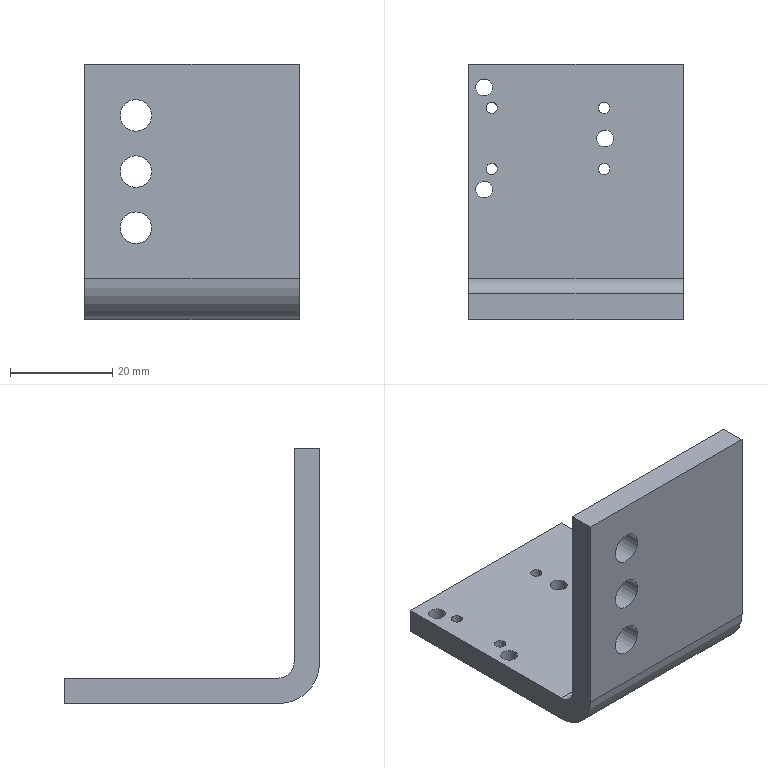Part | NX | features SIMPLE HOLE 10, DATUM_CSYS 5, SKETCH 4, HOLE PACKAGE 3, EXTRUDE 1 | 1 solid | 20 faces | box 42 x 50 x 50 mm | volume 18797 mm3 | cylinder 12 | plane 8 | commonest cylinder face diameters 2.2 x4 3.3 x3 6.2 x3 6 x1 16 x1
STEP:
#1=CARTESIAN_POINT('',(-11.,0.,43.1));
#2=VERTEX_POINT('',#1);
#3=CARTESIAN_POINT('',(-11.,0.,40.));
#4=DIRECTION('',(0.,1.,0.));
#5=DIRECTION('',(0.,0.,1.));
#6=AXIS2_PLACEMENT_3D('',#3,#4,#5);
#7=CIRCLE('',#6,3.1);
#8=EDGE_CURVE('',#2,#2,#7,.T.);
#9=ORIENTED_EDGE('',*,*,#8,.T.);
#10=EDGE_LOOP('',(#9));
#11=FACE_BOUND('',#10,.T.);
#12=CARTESIAN_POINT('',(-11.,0.,32.1));
#13=VERTEX_POINT('',#12);
#14=CARTESIAN_POINT('',(-11.,0.,29.));
#15=DIRECTION('',(0.,1.,0.));
#16=DIRECTION('',(0.,0.,1.));
#17=AXIS2_PLACEMENT_3D('',#14,#15,#16);
#18=CIRCLE('',#17,3.1);
#19=EDGE_CURVE('',#13,#13,#18,.T.);
#20=ORIENTED_EDGE('',*,*,#19,.T.);
#21=EDGE_LOOP('',(#20));
#22=FACE_BOUND('',#21,.T.);
#23=CARTESIAN_POINT('',(-11.,0.,21.1));
#24=VERTEX_POINT('',#23);
#25=CARTESIAN_POINT('',(-11.,0.,18.));
#26=DIRECTION('',(0.,1.,0.));
#27=DIRECTION('',(0.,0.,1.));
#28=AXIS2_PLACEMENT_3D('',#25,#26,#27);
#29=CIRCLE('',#28,3.1);
#30=EDGE_CURVE('',#24,#24,#29,.T.);
#31=ORIENTED_EDGE('',*,*,#30,.T.);
#32=EDGE_LOOP('',(#31));
#33=FACE_BOUND('',#32,.T.);
#34=CARTESIAN_POINT('',(-21.,0.,50.));
#35=VERTEX_POINT('',#34);
#36=CARTESIAN_POINT('',(-21.,0.,8.));
#37=VERTEX_POINT('',#36);
#38=CARTESIAN_POINT('',(-21.,0.,50.));
#39=DIRECTION('',(0.,0.,-1.));
#40=VECTOR('',#39,1000.);
#41=LINE('',#38,#40);
#42=EDGE_CURVE('',#35,#37,#41,.T.);
#43=ORIENTED_EDGE('',*,*,#42,.T.);
#44=CARTESIAN_POINT('',(21.,0.,8.));
#45=VERTEX_POINT('',#44);
#46=CARTESIAN_POINT('',(21.,0.,8.));
#47=DIRECTION('',(-1.,0.,0.));
#48=VECTOR('',#47,1000.);
#49=LINE('',#46,#48);
#50=EDGE_CURVE('',#45,#37,#49,.T.);
#51=ORIENTED_EDGE('',*,*,#50,.F.);
#52=CARTESIAN_POINT('',(21.,0.,50.));
#53=VERTEX_POINT('',#52);
#54=CARTESIAN_POINT('',(21.,0.,50.));
#55=DIRECTION('',(0.,0.,-1.));
#56=VECTOR('',#55,1000.);
#57=LINE('',#54,#56);
#58=EDGE_CURVE('',#53,#45,#57,.T.);
#59=ORIENTED_EDGE('',*,*,#58,.F.);
#60=CARTESIAN_POINT('',(21.,0.,50.));
#61=DIRECTION('',(-1.,0.,0.));
#62=VECTOR('',#61,1000.);
#63=LINE('',#60,#62);
#64=EDGE_CURVE('',#53,#35,#63,.T.);
#65=ORIENTED_EDGE('',*,*,#64,.T.);
#66=EDGE_LOOP('',(#43,#51,#59,#65));
#67=FACE_BOUND('',#66,.T.);
#68=CARTESIAN_POINT('',(21.,0.,50.));
#69=DIRECTION('',(0.,1.,0.));
#70=DIRECTION('',(0.,0.,1.));
#71=AXIS2_PLACEMENT_3D('',#68,#69,#70);
#72=PLANE('',#71);
#73=ADVANCED_FACE('',(#11,#22,#33,#67),#72,.F.);
#74=CARTESIAN_POINT('',(-21.,8.,0.));
#75=VERTEX_POINT('',#74);
#76=CARTESIAN_POINT('',(-21.,8.,8.));
#77=DIRECTION('',(1.,0.,0.));
#78=DIRECTION('',(0.,1.,0.));
#79=AXIS2_PLACEMENT_3D('',#76,#77,#78);
#80=CIRCLE('',#79,8.);
#81=EDGE_CURVE('',#37,#75,#80,.T.);
#82=ORIENTED_EDGE('',*,*,#81,.T.);
#83=CARTESIAN_POINT('',(21.,8.,0.));
#84=VERTEX_POINT('',#83);
#85=CARTESIAN_POINT('',(21.,8.,0.));
#86=DIRECTION('',(-1.,0.,0.));
#87=VECTOR('',#86,1000.);
#88=LINE('',#85,#87);
#89=EDGE_CURVE('',#84,#75,#88,.T.);
#90=ORIENTED_EDGE('',*,*,#89,.F.);
#91=CARTESIAN_POINT('',(21.,8.,8.));
#92=DIRECTION('',(1.,0.,0.));
#93=DIRECTION('',(0.,1.,0.));
#94=AXIS2_PLACEMENT_3D('',#91,#92,#93);
#95=CIRCLE('',#94,8.);
#96=EDGE_CURVE('',#45,#84,#95,.T.);
#97=ORIENTED_EDGE('',*,*,#96,.F.);
#98=ORIENTED_EDGE('',*,*,#50,.T.);
#99=EDGE_LOOP('',(#82,#90,#97,#98));
#100=FACE_BOUND('',#99,.T.);
#101=CARTESIAN_POINT('',(21.,8.,8.));
#102=DIRECTION('',(-1.,0.,0.));
#103=DIRECTION('',(0.,0.,1.));
#104=AXIS2_PLACEMENT_3D('',#101,#102,#103);
#105=CYLINDRICAL_SURFACE('',#104,8.);
#106=ADVANCED_FACE('',(#100),#105,.T.);
#107=CARTESIAN_POINT('',(6.6,41.5,0.));
#108=VERTEX_POINT('',#107);
#109=CARTESIAN_POINT('',(5.5,41.5,0.));
#110=DIRECTION('',(0.,0.,1.));
#111=DIRECTION('',(1.,0.,0.));
#112=AXIS2_PLACEMENT_3D('',#109,#110,#111);
#113=CIRCLE('',#112,1.1);
#114=EDGE_CURVE('',#108,#108,#113,.T.);
#115=ORIENTED_EDGE('',*,*,#114,.T.);
#116=EDGE_LOOP('',(#115));
#117=FACE_BOUND('',#116,.T.);
#118=CARTESIAN_POINT('',(6.6,29.5,0.));
#119=VERTEX_POINT('',#118);
#120=CARTESIAN_POINT('',(5.5,29.5,0.));
#121=DIRECTION('',(0.,0.,1.));
#122=DIRECTION('',(1.,0.,0.));
#123=AXIS2_PLACEMENT_3D('',#120,#121,#122);
#124=CIRCLE('',#123,1.1);
#125=EDGE_CURVE('',#119,#119,#124,.T.);
#126=ORIENTED_EDGE('',*,*,#125,.T.);
#127=EDGE_LOOP('',(#126));
#128=FACE_BOUND('',#127,.T.);
#129=CARTESIAN_POINT('',(-15.4,41.5,0.));
#130=VERTEX_POINT('',#129);
#131=CARTESIAN_POINT('',(-16.5,41.5,0.));
#132=DIRECTION('',(0.,0.,1.));
#133=DIRECTION('',(1.,0.,0.));
#134=AXIS2_PLACEMENT_3D('',#131,#132,#133);
#135=CIRCLE('',#134,1.1);
#136=EDGE_CURVE('',#130,#130,#135,.T.);
#137=ORIENTED_EDGE('',*,*,#136,.T.);
#138=EDGE_LOOP('',(#137));
#139=FACE_BOUND('',#138,.T.);
#140=CARTESIAN_POINT('',(-15.4,29.5,0.));
#141=VERTEX_POINT('',#140);
#142=CARTESIAN_POINT('',(-16.5,29.5,0.));
#143=DIRECTION('',(0.,0.,1.));
#144=DIRECTION('',(1.,0.,0.));
#145=AXIS2_PLACEMENT_3D('',#142,#143,#144);
#146=CIRCLE('',#145,1.1);
#147=EDGE_CURVE('',#141,#141,#146,.T.);
#148=ORIENTED_EDGE('',*,*,#147,.T.);
#149=EDGE_LOOP('',(#148));
#150=FACE_BOUND('',#149,.T.);
#151=CARTESIAN_POINT('',(7.35,35.5,0.));
#152=VERTEX_POINT('',#151);
#153=CARTESIAN_POINT('',(5.7,35.5,0.));
#154=DIRECTION('',(0.,0.,1.));
#155=DIRECTION('',(1.,0.,0.));
#156=AXIS2_PLACEMENT_3D('',#153,#154,#155);
#157=CIRCLE('',#156,1.65);
#158=EDGE_CURVE('',#152,#152,#157,.T.);
#159=ORIENTED_EDGE('',*,*,#158,.T.);
#160=EDGE_LOOP('',(#159));
#161=FACE_BOUND('',#160,.T.);
#162=CARTESIAN_POINT('',(-16.35,45.5,0.));
#163=VERTEX_POINT('',#162);
#164=CARTESIAN_POINT('',(-18.,45.5,0.));
#165=DIRECTION('',(0.,0.,1.));
#166=DIRECTION('',(1.,0.,0.));
#167=AXIS2_PLACEMENT_3D('',#164,#165,#166);
#168=CIRCLE('',#167,1.65);
#169=EDGE_CURVE('',#163,#163,#168,.T.);
#170=ORIENTED_EDGE('',*,*,#169,.T.);
#171=EDGE_LOOP('',(#170));
#172=FACE_BOUND('',#171,.T.);
#173=CARTESIAN_POINT('',(-16.35,25.5,0.));
#174=VERTEX_POINT('',#173);
#175=CARTESIAN_POINT('',(-18.,25.5,0.));
#176=DIRECTION('',(0.,0.,1.));
#177=DIRECTION('',(1.,0.,0.));
#178=AXIS2_PLACEMENT_3D('',#175,#176,#177);
#179=CIRCLE('',#178,1.65);
#180=EDGE_CURVE('',#174,#174,#179,.T.);
#181=ORIENTED_EDGE('',*,*,#180,.T.);
#182=EDGE_LOOP('',(#181));
#183=FACE_BOUND('',#182,.T.);
#184=CARTESIAN_POINT('',(-21.,50.,0.));
#185=VERTEX_POINT('',#184);
#186=CARTESIAN_POINT('',(-21.,8.,0.));
#187=DIRECTION('',(0.,1.,0.));
#188=VECTOR('',#187,1000.);
#189=LINE('',#186,#188);
#190=EDGE_CURVE('',#75,#185,#189,.T.);
#191=ORIENTED_EDGE('',*,*,#190,.T.);
#192=CARTESIAN_POINT('',(21.,50.,0.));
#193=VERTEX_POINT('',#192);
#194=CARTESIAN_POINT('',(21.,50.,0.));
#195=DIRECTION('',(-1.,0.,0.));
#196=VECTOR('',#195,1000.);
#197=LINE('',#194,#196);
#198=EDGE_CURVE('',#193,#185,#197,.T.);
#199=ORIENTED_EDGE('',*,*,#198,.F.);
#200=CARTESIAN_POINT('',(21.,8.,0.));
#201=DIRECTION('',(0.,1.,0.));
#202=VECTOR('',#201,1000.);
#203=LINE('',#200,#202);
#204=EDGE_CURVE('',#84,#193,#203,.T.);
#205=ORIENTED_EDGE('',*,*,#204,.F.);
#206=ORIENTED_EDGE('',*,*,#89,.T.);
#207=EDGE_LOOP('',(#191,#199,#205,#206));
#208=FACE_BOUND('',#207,.T.);
#209=CARTESIAN_POINT('',(21.,8.,0.));
#210=DIRECTION('',(0.,0.,1.));
#211=DIRECTION('',(1.,0.,0.));
#212=AXIS2_PLACEMENT_3D('',#209,#210,#211);
#213=PLANE('',#212);
#214=ADVANCED_FACE('',(#117,#128,#139,#150,#161,#172,#183,#208),#213,.F.);
#215=CARTESIAN_POINT('',(-21.,50.,5.));
#216=VERTEX_POINT('',#215);
#217=CARTESIAN_POINT('',(-21.,50.,0.));
#218=DIRECTION('',(0.,0.,1.));
#219=VECTOR('',#218,1000.);
#220=LINE('',#217,#219);
#221=EDGE_CURVE('',#185,#216,#220,.T.);
#222=ORIENTED_EDGE('',*,*,#221,.T.);
#223=CARTESIAN_POINT('',(21.,50.,5.));
#224=VERTEX_POINT('',#223);
#225=CARTESIAN_POINT('',(21.,50.,5.));
#226=DIRECTION('',(-1.,0.,0.));
#227=VECTOR('',#226,1000.);
#228=LINE('',#225,#227);
#229=EDGE_CURVE('',#224,#216,#228,.T.);
#230=ORIENTED_EDGE('',*,*,#229,.F.);
#231=CARTESIAN_POINT('',(21.,50.,0.));
#232=DIRECTION('',(0.,0.,1.));
#233=VECTOR('',#232,1000.);
#234=LINE('',#231,#233);
#235=EDGE_CURVE('',#193,#224,#234,.T.);
#236=ORIENTED_EDGE('',*,*,#235,.F.);
#237=ORIENTED_EDGE('',*,*,#198,.T.);
#238=EDGE_LOOP('',(#222,#230,#236,#237));
#239=FACE_BOUND('',#238,.T.);
#240=CARTESIAN_POINT('',(21.,50.,0.));
#241=DIRECTION('',(0.,-1.,0.));
#242=DIRECTION('',(0.,0.,-1.));
#243=AXIS2_PLACEMENT_3D('',#240,#241,#242);
#244=PLANE('',#243);
#245=ADVANCED_FACE('',(#239),#244,.F.);
#246=CARTESIAN_POINT('',(5.5,42.6,5.));
#247=VERTEX_POINT('',#246);
#248=CARTESIAN_POINT('',(5.5,41.5,5.));
#249=DIRECTION('',(0.,0.,-1.));
#250=DIRECTION('',(0.,1.,0.));
#251=AXIS2_PLACEMENT_3D('',#248,#249,#250);
#252=CIRCLE('',#251,1.1);
#253=EDGE_CURVE('',#247,#247,#252,.T.);
#254=ORIENTED_EDGE('',*,*,#253,.T.);
#255=EDGE_LOOP('',(#254));
#256=FACE_BOUND('',#255,.T.);
#257=CARTESIAN_POINT('',(5.5,30.6,5.));
#258=VERTEX_POINT('',#257);
#259=CARTESIAN_POINT('',(5.5,29.5,5.));
#260=DIRECTION('',(0.,0.,-1.));
#261=DIRECTION('',(0.,1.,0.));
#262=AXIS2_PLACEMENT_3D('',#259,#260,#261);
#263=CIRCLE('',#262,1.1);
#264=EDGE_CURVE('',#258,#258,#263,.T.);
#265=ORIENTED_EDGE('',*,*,#264,.T.);
#266=EDGE_LOOP('',(#265));
#267=FACE_BOUND('',#266,.T.);
#268=CARTESIAN_POINT('',(-16.5,42.6,5.));
#269=VERTEX_POINT('',#268);
#270=CARTESIAN_POINT('',(-16.5,41.5,5.));
#271=DIRECTION('',(0.,0.,-1.));
#272=DIRECTION('',(0.,1.,0.));
#273=AXIS2_PLACEMENT_3D('',#270,#271,#272);
#274=CIRCLE('',#273,1.1);
#275=EDGE_CURVE('',#269,#269,#274,.T.);
#276=ORIENTED_EDGE('',*,*,#275,.T.);
#277=EDGE_LOOP('',(#276));
#278=FACE_BOUND('',#277,.T.);
#279=CARTESIAN_POINT('',(-16.5,30.6,5.));
#280=VERTEX_POINT('',#279);
#281=CARTESIAN_POINT('',(-16.5,29.5,5.));
#282=DIRECTION('',(0.,0.,-1.));
#283=DIRECTION('',(0.,1.,0.));
#284=AXIS2_PLACEMENT_3D('',#281,#282,#283);
#285=CIRCLE('',#284,1.1);
#286=EDGE_CURVE('',#280,#280,#285,.T.);
#287=ORIENTED_EDGE('',*,*,#286,.T.);
#288=EDGE_LOOP('',(#287));
#289=FACE_BOUND('',#288,.T.);
#290=CARTESIAN_POINT('',(5.7,37.15,5.));
#291=VERTEX_POINT('',#290);
#292=CARTESIAN_POINT('',(5.7,35.5,5.));
#293=DIRECTION('',(0.,0.,-1.));
#294=DIRECTION('',(0.,1.,0.));
#295=AXIS2_PLACEMENT_3D('',#292,#293,#294);
#296=CIRCLE('',#295,1.65);
#297=EDGE_CURVE('',#291,#291,#296,.T.);
#298=ORIENTED_EDGE('',*,*,#297,.T.);
#299=EDGE_LOOP('',(#298));
#300=FACE_BOUND('',#299,.T.);
#301=CARTESIAN_POINT('',(-18.,47.15,5.));
#302=VERTEX_POINT('',#301);
#303=CARTESIAN_POINT('',(-18.,45.5,5.));
#304=DIRECTION('',(0.,0.,-1.));
#305=DIRECTION('',(0.,1.,0.));
#306=AXIS2_PLACEMENT_3D('',#303,#304,#305);
#307=CIRCLE('',#306,1.65);
#308=EDGE_CURVE('',#302,#302,#307,.T.);
#309=ORIENTED_EDGE('',*,*,#308,.T.);
#310=EDGE_LOOP('',(#309));
#311=FACE_BOUND('',#310,.T.);
#312=CARTESIAN_POINT('',(-18.,27.15,5.));
#313=VERTEX_POINT('',#312);
#314=CARTESIAN_POINT('',(-18.,25.5,5.));
#315=DIRECTION('',(0.,0.,-1.));
#316=DIRECTION('',(0.,1.,0.));
#317=AXIS2_PLACEMENT_3D('',#314,#315,#316);
#318=CIRCLE('',#317,1.65);
#319=EDGE_CURVE('',#313,#313,#318,.T.);
#320=ORIENTED_EDGE('',*,*,#319,.T.);
#321=EDGE_LOOP('',(#320));
#322=FACE_BOUND('',#321,.T.);
#323=CARTESIAN_POINT('',(-21.,8.,5.));
#324=VERTEX_POINT('',#323);
#325=CARTESIAN_POINT('',(-21.,50.,5.));
#326=DIRECTION('',(0.,-1.,0.));
#327=VECTOR('',#326,1000.);
#328=LINE('',#325,#327);
#329=EDGE_CURVE('',#216,#324,#328,.T.);
#330=ORIENTED_EDGE('',*,*,#329,.T.);
#331=CARTESIAN_POINT('',(21.,8.,5.));
#332=VERTEX_POINT('',#331);
#333=CARTESIAN_POINT('',(21.,8.,5.));
#334=DIRECTION('',(-1.,0.,0.));
#335=VECTOR('',#334,1000.);
#336=LINE('',#333,#335);
#337=EDGE_CURVE('',#332,#324,#336,.T.);
#338=ORIENTED_EDGE('',*,*,#337,.F.);
#339=CARTESIAN_POINT('',(21.,50.,5.));
#340=DIRECTION('',(0.,-1.,0.));
#341=VECTOR('',#340,1000.);
#342=LINE('',#339,#341);
#343=EDGE_CURVE('',#224,#332,#342,.T.);
#344=ORIENTED_EDGE('',*,*,#343,.F.);
#345=ORIENTED_EDGE('',*,*,#229,.T.);
#346=EDGE_LOOP('',(#330,#338,#344,#345));
#347=FACE_BOUND('',#346,.T.);
#348=CARTESIAN_POINT('',(21.,50.,5.));
#349=DIRECTION('',(0.,0.,-1.));
#350=DIRECTION('',(0.,1.,0.));
#351=AXIS2_PLACEMENT_3D('',#348,#349,#350);
#352=PLANE('',#351);
#353=ADVANCED_FACE('',(#256,#267,#278,#289,#300,#311,#322,#347),#352,.F.);
#354=CARTESIAN_POINT('',(-21.,5.,8.));
#355=VERTEX_POINT('',#354);
#356=CARTESIAN_POINT('',(-21.,8.,8.));
#357=DIRECTION('',(-1.,0.,0.));
#358=DIRECTION('',(0.,1.,0.));
#359=AXIS2_PLACEMENT_3D('',#356,#357,#358);
#360=CIRCLE('',#359,3.);
#361=EDGE_CURVE('',#324,#355,#360,.T.);
#362=ORIENTED_EDGE('',*,*,#361,.T.);
#363=CARTESIAN_POINT('',(21.,5.,8.));
#364=VERTEX_POINT('',#363);
#365=CARTESIAN_POINT('',(21.,5.,8.));
#366=DIRECTION('',(-1.,0.,0.));
#367=VECTOR('',#366,1000.);
#368=LINE('',#365,#367);
#369=EDGE_CURVE('',#364,#355,#368,.T.);
#370=ORIENTED_EDGE('',*,*,#369,.F.);
#371=CARTESIAN_POINT('',(21.,8.,8.));
#372=DIRECTION('',(-1.,0.,0.));
#373=DIRECTION('',(0.,1.,0.));
#374=AXIS2_PLACEMENT_3D('',#371,#372,#373);
#375=CIRCLE('',#374,3.);
#376=EDGE_CURVE('',#332,#364,#375,.T.);
#377=ORIENTED_EDGE('',*,*,#376,.F.);
#378=ORIENTED_EDGE('',*,*,#337,.T.);
#379=EDGE_LOOP('',(#362,#370,#377,#378));
#380=FACE_BOUND('',#379,.T.);
#381=CARTESIAN_POINT('',(21.,8.,8.));
#382=DIRECTION('',(-1.,0.,0.));
#383=DIRECTION('',(0.,0.,1.));
#384=AXIS2_PLACEMENT_3D('',#381,#382,#383);
#385=CYLINDRICAL_SURFACE('',#384,3.);
#386=ADVANCED_FACE('',(#380),#385,.F.);
#387=CARTESIAN_POINT('',(-11.,5.,36.9));
#388=VERTEX_POINT('',#387);
#389=CARTESIAN_POINT('',(-11.,5.,40.));
#390=DIRECTION('',(0.,-1.,0.));
#391=DIRECTION('',(0.,0.,-1.));
#392=AXIS2_PLACEMENT_3D('',#389,#390,#391);
#393=CIRCLE('',#392,3.1);
#394=EDGE_CURVE('',#388,#388,#393,.T.);
#395=ORIENTED_EDGE('',*,*,#394,.T.);
#396=EDGE_LOOP('',(#395));
#397=FACE_BOUND('',#396,.T.);
#398=CARTESIAN_POINT('',(-11.,5.,25.9));
#399=VERTEX_POINT('',#398);
#400=CARTESIAN_POINT('',(-11.,5.,29.));
#401=DIRECTION('',(0.,-1.,0.));
#402=DIRECTION('',(0.,0.,-1.));
#403=AXIS2_PLACEMENT_3D('',#400,#401,#402);
#404=CIRCLE('',#403,3.1);
#405=EDGE_CURVE('',#399,#399,#404,.T.);
#406=ORIENTED_EDGE('',*,*,#405,.T.);
#407=EDGE_LOOP('',(#406));
#408=FACE_BOUND('',#407,.T.);
#409=CARTESIAN_POINT('',(-11.,5.,14.9));
#410=VERTEX_POINT('',#409);
#411=CARTESIAN_POINT('',(-11.,5.,18.));
#412=DIRECTION('',(0.,-1.,0.));
#413=DIRECTION('',(0.,0.,-1.));
#414=AXIS2_PLACEMENT_3D('',#411,#412,#413);
#415=CIRCLE('',#414,3.1);
#416=EDGE_CURVE('',#410,#410,#415,.T.);
#417=ORIENTED_EDGE('',*,*,#416,.T.);
#418=EDGE_LOOP('',(#417));
#419=FACE_BOUND('',#418,.T.);
#420=CARTESIAN_POINT('',(-21.,5.,50.));
#421=VERTEX_POINT('',#420);
#422=CARTESIAN_POINT('',(-21.,5.,8.));
#423=DIRECTION('',(0.,0.,1.));
#424=VECTOR('',#423,1000.);
#425=LINE('',#422,#424);
#426=EDGE_CURVE('',#355,#421,#425,.T.);
#427=ORIENTED_EDGE('',*,*,#426,.T.);
#428=CARTESIAN_POINT('',(21.,5.,50.));
#429=VERTEX_POINT('',#428);
#430=CARTESIAN_POINT('',(21.,5.,50.));
#431=DIRECTION('',(-1.,0.,0.));
#432=VECTOR('',#431,1000.);
#433=LINE('',#430,#432);
#434=EDGE_CURVE('',#429,#421,#433,.T.);
#435=ORIENTED_EDGE('',*,*,#434,.F.);
#436=CARTESIAN_POINT('',(21.,5.,8.));
#437=DIRECTION('',(0.,0.,1.));
#438=VECTOR('',#437,1000.);
#439=LINE('',#436,#438);
#440=EDGE_CURVE('',#364,#429,#439,.T.);
#441=ORIENTED_EDGE('',*,*,#440,.F.);
#442=ORIENTED_EDGE('',*,*,#369,.T.);
#443=EDGE_LOOP('',(#427,#435,#441,#442));
#444=FACE_BOUND('',#443,.T.);
#445=CARTESIAN_POINT('',(21.,5.,8.));
#446=DIRECTION('',(0.,-1.,0.));
#447=DIRECTION('',(0.,0.,-1.));
#448=AXIS2_PLACEMENT_3D('',#445,#446,#447);
#449=PLANE('',#448);
#450=ADVANCED_FACE('',(#397,#408,#419,#444),#449,.F.);
#451=CARTESIAN_POINT('',(-21.,5.,50.));
#452=DIRECTION('',(0.,-1.,0.));
#453=VECTOR('',#452,1000.);
#454=LINE('',#451,#453);
#455=EDGE_CURVE('',#421,#35,#454,.T.);
#456=ORIENTED_EDGE('',*,*,#455,.T.);
#457=ORIENTED_EDGE('',*,*,#64,.F.);
#458=CARTESIAN_POINT('',(21.,5.,50.));
#459=DIRECTION('',(0.,-1.,0.));
#460=VECTOR('',#459,1000.);
#461=LINE('',#458,#460);
#462=EDGE_CURVE('',#429,#53,#461,.T.);
#463=ORIENTED_EDGE('',*,*,#462,.F.);
#464=ORIENTED_EDGE('',*,*,#434,.T.);
#465=EDGE_LOOP('',(#456,#457,#463,#464));
#466=FACE_BOUND('',#465,.T.);
#467=CARTESIAN_POINT('',(21.,5.,50.));
#468=DIRECTION('',(0.,0.,-1.));
#469=DIRECTION('',(-1.,0.,0.));
#470=AXIS2_PLACEMENT_3D('',#467,#468,#469);
#471=PLANE('',#470);
#472=ADVANCED_FACE('',(#466),#471,.F.);
#473=ORIENTED_EDGE('',*,*,#58,.T.);
#474=ORIENTED_EDGE('',*,*,#96,.T.);
#475=ORIENTED_EDGE('',*,*,#204,.T.);
#476=ORIENTED_EDGE('',*,*,#235,.T.);
#477=ORIENTED_EDGE('',*,*,#343,.T.);
#478=ORIENTED_EDGE('',*,*,#376,.T.);
#479=ORIENTED_EDGE('',*,*,#440,.T.);
#480=ORIENTED_EDGE('',*,*,#462,.T.);
#481=EDGE_LOOP('',(#473,#474,#475,#476,#477,#478,#479,#480));
#482=FACE_BOUND('',#481,.T.);
#483=CARTESIAN_POINT('',(21.,8.,8.));
#484=DIRECTION('',(1.,0.,0.));
#485=DIRECTION('',(0.,0.,-1.));
#486=AXIS2_PLACEMENT_3D('',#483,#484,#485);
#487=PLANE('',#486);
#488=ADVANCED_FACE('',(#482),#487,.T.);
#489=ORIENTED_EDGE('',*,*,#42,.F.);
#490=ORIENTED_EDGE('',*,*,#455,.F.);
#491=ORIENTED_EDGE('',*,*,#426,.F.);
#492=ORIENTED_EDGE('',*,*,#361,.F.);
#493=ORIENTED_EDGE('',*,*,#329,.F.);
#494=ORIENTED_EDGE('',*,*,#221,.F.);
#495=ORIENTED_EDGE('',*,*,#190,.F.);
#496=ORIENTED_EDGE('',*,*,#81,.F.);
#497=EDGE_LOOP('',(#489,#490,#491,#492,#493,#494,#495,#496));
#498=FACE_BOUND('',#497,.T.);
#499=CARTESIAN_POINT('',(-21.,8.,8.));
#500=DIRECTION('',(1.,0.,0.));
#501=DIRECTION('',(0.,0.,-1.));
#502=AXIS2_PLACEMENT_3D('',#499,#500,#501);
#503=PLANE('',#502);
#504=ADVANCED_FACE('',(#498),#503,.F.);
#505=ORIENTED_EDGE('',*,*,#416,.F.);
#506=EDGE_LOOP('',(#505));
#507=FACE_BOUND('',#506,.T.);
#508=ORIENTED_EDGE('',*,*,#30,.F.);
#509=EDGE_LOOP('',(#508));
#510=FACE_BOUND('',#509,.T.);
#511=CARTESIAN_POINT('',(-11.,5.,18.));
#512=DIRECTION('',(0.,-1.,0.));
#513=DIRECTION('',(0.,0.,-1.));
#514=AXIS2_PLACEMENT_3D('',#511,#512,#513);
#515=CYLINDRICAL_SURFACE('',#514,3.1);
#516=ADVANCED_FACE('',(#507,#510),#515,.F.);
#517=ORIENTED_EDGE('',*,*,#405,.F.);
#518=EDGE_LOOP('',(#517));
#519=FACE_BOUND('',#518,.T.);
#520=ORIENTED_EDGE('',*,*,#19,.F.);
#521=EDGE_LOOP('',(#520));
#522=FACE_BOUND('',#521,.T.);
#523=CARTESIAN_POINT('',(-11.,5.,29.));
#524=DIRECTION('',(0.,-1.,0.));
#525=DIRECTION('',(0.,0.,-1.));
#526=AXIS2_PLACEMENT_3D('',#523,#524,#525);
#527=CYLINDRICAL_SURFACE('',#526,3.1);
#528=ADVANCED_FACE('',(#519,#522),#527,.F.);
#529=ORIENTED_EDGE('',*,*,#394,.F.);
#530=EDGE_LOOP('',(#529));
#531=FACE_BOUND('',#530,.T.);
#532=ORIENTED_EDGE('',*,*,#8,.F.);
#533=EDGE_LOOP('',(#532));
#534=FACE_BOUND('',#533,.T.);
#535=CARTESIAN_POINT('',(-11.,5.,40.));
#536=DIRECTION('',(0.,-1.,0.));
#537=DIRECTION('',(0.,0.,-1.));
#538=AXIS2_PLACEMENT_3D('',#535,#536,#537);
#539=CYLINDRICAL_SURFACE('',#538,3.1);
#540=ADVANCED_FACE('',(#531,#534),#539,.F.);
#541=ORIENTED_EDGE('',*,*,#180,.F.);
#542=EDGE_LOOP('',(#541));
#543=FACE_BOUND('',#542,.T.);
#544=ORIENTED_EDGE('',*,*,#319,.F.);
#545=EDGE_LOOP('',(#544));
#546=FACE_BOUND('',#545,.T.);
#547=CARTESIAN_POINT('',(-18.,25.5,0.));
#548=DIRECTION('',(0.,0.,1.));
#549=DIRECTION('',(1.,0.,0.));
#550=AXIS2_PLACEMENT_3D('',#547,#548,#549);
#551=CYLINDRICAL_SURFACE('',#550,1.65);
#552=ADVANCED_FACE('',(#543,#546),#551,.F.);
#553=ORIENTED_EDGE('',*,*,#169,.F.);
#554=EDGE_LOOP('',(#553));
#555=FACE_BOUND('',#554,.T.);
#556=ORIENTED_EDGE('',*,*,#308,.F.);
#557=EDGE_LOOP('',(#556));
#558=FACE_BOUND('',#557,.T.);
#559=CARTESIAN_POINT('',(-18.,45.5,0.));
#560=DIRECTION('',(0.,0.,1.));
#561=DIRECTION('',(1.,0.,0.));
#562=AXIS2_PLACEMENT_3D('',#559,#560,#561);
#563=CYLINDRICAL_SURFACE('',#562,1.65);
#564=ADVANCED_FACE('',(#555,#558),#563,.F.);
#565=ORIENTED_EDGE('',*,*,#158,.F.);
#566=EDGE_LOOP('',(#565));
#567=FACE_BOUND('',#566,.T.);
#568=ORIENTED_EDGE('',*,*,#297,.F.);
#569=EDGE_LOOP('',(#568));
#570=FACE_BOUND('',#569,.T.);
#571=CARTESIAN_POINT('',(5.7,35.5,0.));
#572=DIRECTION('',(0.,0.,1.));
#573=DIRECTION('',(1.,0.,0.));
#574=AXIS2_PLACEMENT_3D('',#571,#572,#573);
#575=CYLINDRICAL_SURFACE('',#574,1.65);
#576=ADVANCED_FACE('',(#567,#570),#575,.F.);
#577=ORIENTED_EDGE('',*,*,#147,.F.);
#578=EDGE_LOOP('',(#577));
#579=FACE_BOUND('',#578,.T.);
#580=ORIENTED_EDGE('',*,*,#286,.F.);
#581=EDGE_LOOP('',(#580));
#582=FACE_BOUND('',#581,.T.);
#583=CARTESIAN_POINT('',(-16.5,29.5,0.));
#584=DIRECTION('',(0.,0.,1.));
#585=DIRECTION('',(1.,0.,0.));
#586=AXIS2_PLACEMENT_3D('',#583,#584,#585);
#587=CYLINDRICAL_SURFACE('',#586,1.1);
#588=ADVANCED_FACE('',(#579,#582),#587,.F.);
#589=ORIENTED_EDGE('',*,*,#136,.F.);
#590=EDGE_LOOP('',(#589));
#591=FACE_BOUND('',#590,.T.);
#592=ORIENTED_EDGE('',*,*,#275,.F.);
#593=EDGE_LOOP('',(#592));
#594=FACE_BOUND('',#593,.T.);
#595=CARTESIAN_POINT('',(-16.5,41.5,0.));
#596=DIRECTION('',(0.,0.,1.));
#597=DIRECTION('',(1.,0.,0.));
#598=AXIS2_PLACEMENT_3D('',#595,#596,#597);
#599=CYLINDRICAL_SURFACE('',#598,1.1);
#600=ADVANCED_FACE('',(#591,#594),#599,.F.);
#601=ORIENTED_EDGE('',*,*,#125,.F.);
#602=EDGE_LOOP('',(#601));
#603=FACE_BOUND('',#602,.T.);
#604=ORIENTED_EDGE('',*,*,#264,.F.);
#605=EDGE_LOOP('',(#604));
#606=FACE_BOUND('',#605,.T.);
#607=CARTESIAN_POINT('',(5.5,29.5,0.));
#608=DIRECTION('',(0.,0.,1.));
#609=DIRECTION('',(1.,0.,0.));
#610=AXIS2_PLACEMENT_3D('',#607,#608,#609);
#611=CYLINDRICAL_SURFACE('',#610,1.1);
#612=ADVANCED_FACE('',(#603,#606),#611,.F.);
#613=ORIENTED_EDGE('',*,*,#114,.F.);
#614=EDGE_LOOP('',(#613));
#615=FACE_BOUND('',#614,.T.);
#616=ORIENTED_EDGE('',*,*,#253,.F.);
#617=EDGE_LOOP('',(#616));
#618=FACE_BOUND('',#617,.T.);
#619=CARTESIAN_POINT('',(5.5,41.5,0.));
#620=DIRECTION('',(0.,0.,1.));
#621=DIRECTION('',(1.,0.,0.));
#622=AXIS2_PLACEMENT_3D('',#619,#620,#621);
#623=CYLINDRICAL_SURFACE('',#622,1.1);
#624=ADVANCED_FACE('',(#615,#618),#623,.F.);
#625=CLOSED_SHELL('',(#73,#106,#214,#245,#353,#386,#450,#472,#488,#504,#516,#528,#540,#552,#564,#576,#588,#600,#612,#624));
#626=MANIFOLD_SOLID_BREP('',#625);
#627=(LENGTH_UNIT()NAMED_UNIT(*)SI_UNIT(.MILLI.,.METRE.));
#628=UNCERTAINTY_MEASURE_WITH_UNIT(LENGTH_MEASURE(0.00001),#627,'','');
#629=(NAMED_UNIT(*)PLANE_ANGLE_UNIT()SI_UNIT($,.RADIAN.));
#630=(NAMED_UNIT(*)SI_UNIT($,.STERADIAN.)SOLID_ANGLE_UNIT());
#631=(GEOMETRIC_REPRESENTATION_CONTEXT(3)GLOBAL_UNCERTAINTY_ASSIGNED_CONTEXT((#628))GLOBAL_UNIT_ASSIGNED_CONTEXT((#627,#629,#630))REPRESENTATION_CONTEXT('',''));
#632=ADVANCED_BREP_SHAPE_REPRESENTATION('',(#626),#631);